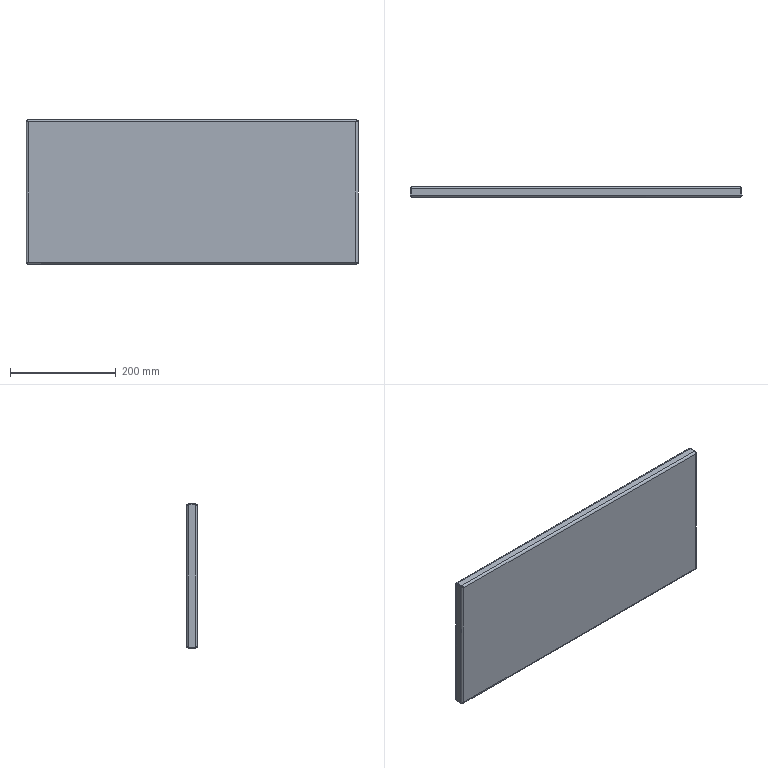Part | SolidWorks | features ICE 3, MirrorPattern 2, FlatPattern 1, SMBaseFlange 1, SMMiteredFlange 1, SheetMetal 1 | 1 solid | 78 faces | box 628 x 20 x 273 mm | volume 459203 mm3 | plane 38 | cylinder 24 | spline 16 | commonest cylinder face diameters 4 x8 7 x8 8 x8